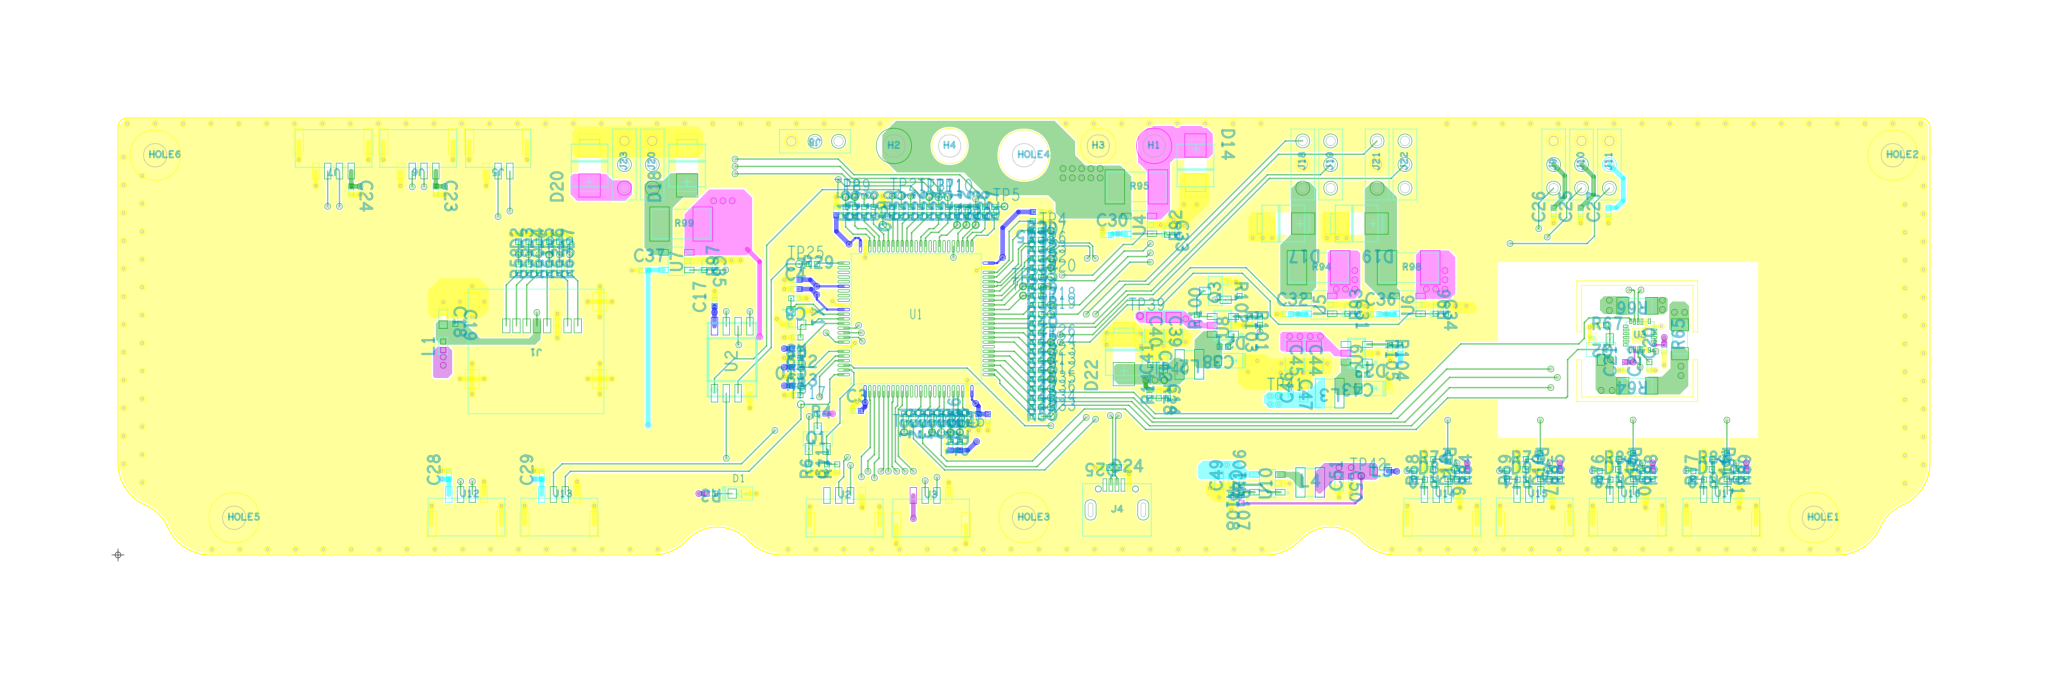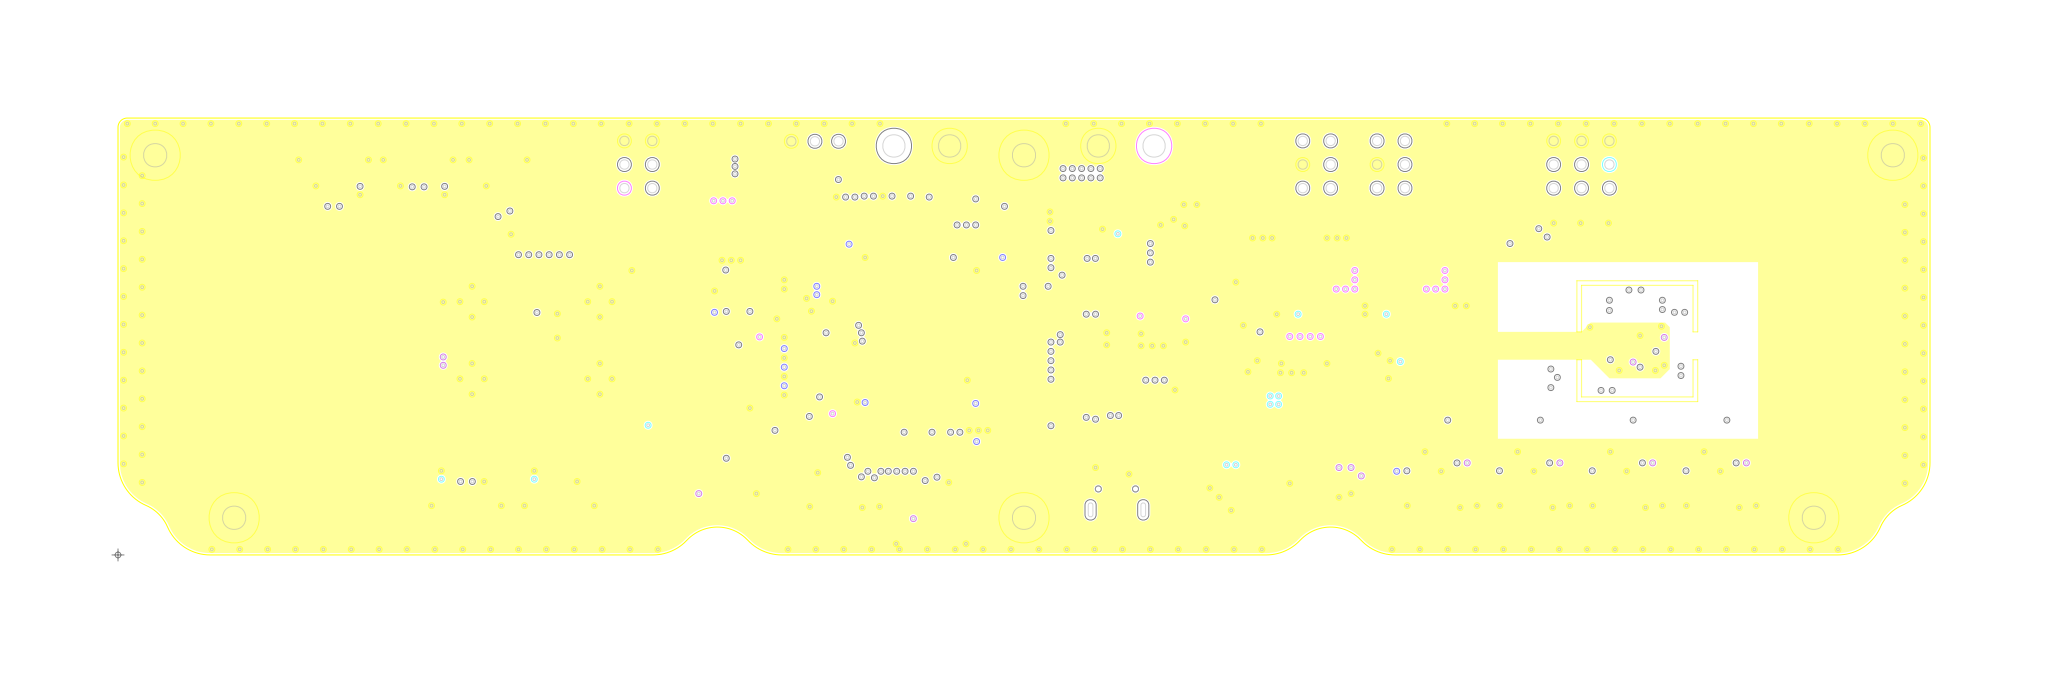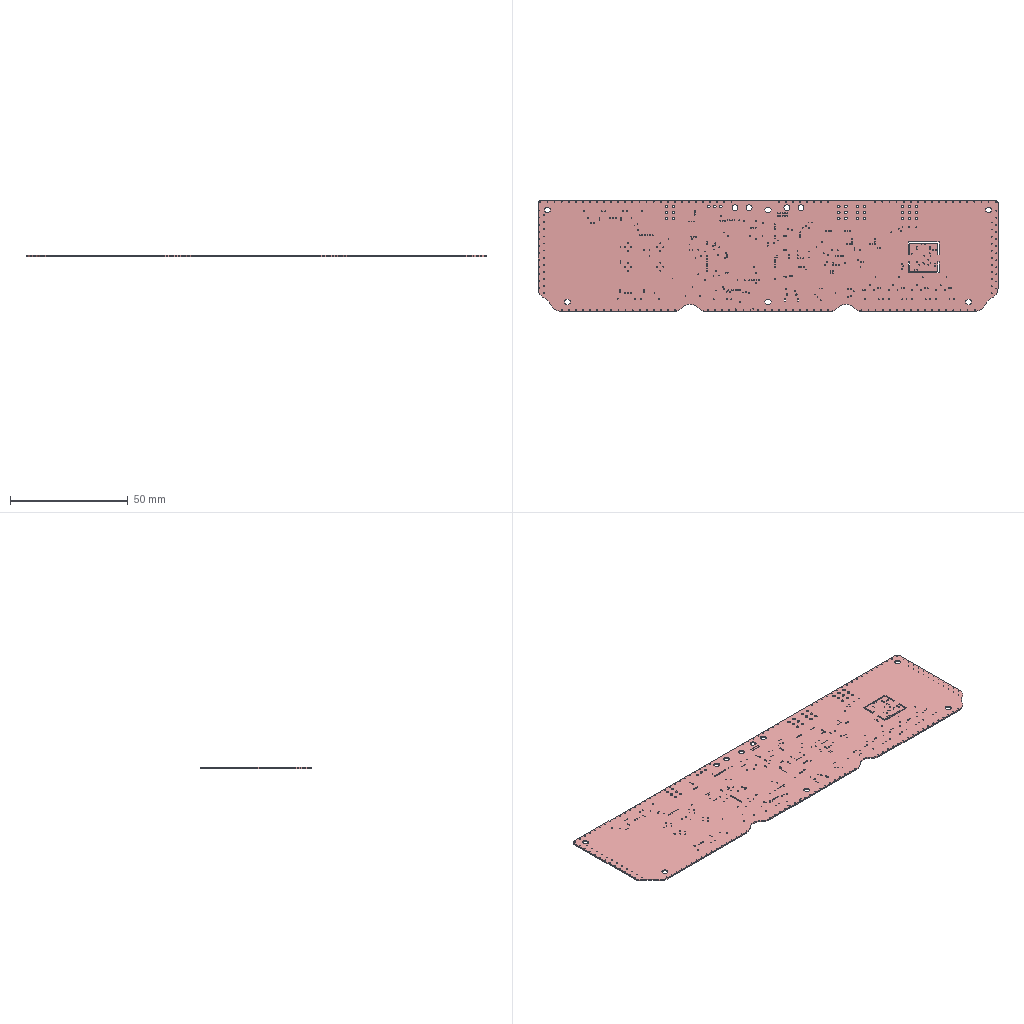Circuit board layout | Cadence Allegro | box 195 x 47 x 0.6 mm
Layer stack:
# Cadence Allegro layer stack of  (unit mm; from the constraint file cross-section; dielectric type: 0 not recorded (Allegro does not mark core vs prepreg), 3 surface material)
index,name,kind,layer,copper_thickness_mm,dielectric_type,dielectric_thickness_mm,dielectric_material,dielectric_constant
0,Top Surface,other,,,,,,
1,TOP,copper,TOP,0.0406,,,,
2,Dielectric1,dielectric,,,0,0.2032,FR-4,4.5
3,L2_GND,copper,L2_GND,0.0305,,,,
4,Dielectric2,dielectric,,,0,0.2032,FR-4,4.5
5,L3_PWR,copper,L3_PWR,0.0305,,,,
6,Dielectric3,dielectric,,,0,0.0889,FR-4,4.5
7,BOTTOM,copper,BOTTOM,0.0406,,,,
8,Bottom Surface,other,,,,,,
# drill layer pairs: low layer,high layer
drill_pair,TOP,BOTTOM
Part placement:
REFDES,COMP_VALUE,SYM_NAME,SYM_X,SYM_Y,SYM_ROTATE,SYM_MIRROR
C1,1uF,C0402,93.6,14.7,90.000,NO
C2,100nF,C0402,98.9,36.9,180.000,NO
C3,100nF,C0402,79.5,15.5,0.000,NO
C4,100nF,C0402,72.9,28.6,0.000,NO
C5,100nF,C0402,77.3,37,270.000,NO
C6,100nF,C0402,92.6,14.7,90.000,NO
C7,100nF,C0402,72.9,29.6,0.000,NO
C8,12pF,C0402,72.9,27.6,180.000,NO
C9,12pF,C0402,73,23.4,180.000,NO
C10,100nF,C0402,73,21.2,180.000,NO
C11,100nF,C0402,77.4,9.3,90.000,NO
C12,100nF,C0402,73,19.2,0.000,NO
C13,100nF,C0402,73,17.2,0.000,NO
C14,100nF,C0402,112,17.3,270.000,NO
C15,2.2uF,C0402,98.9,35.9,180.000,NO
C16,2.2uF,C0402,91.6,14.7,90.000,NO
C17,100nF,C0402,64.2,27.2,90.000,NO
C18,10uF,C0603,35,25.5,270.000,NO
C19,100nF,C0402,36.3,25.3,270.000,NO
C20,100nF,C0402,166.4,22.2,90.000,NO
C21,100nF,C0402,162.2,20.3,90.000,NO
C22,100nF,C0402,164.8,20.3,90.000,NO
C23,100nF,C0402,34.2,39.2,270.000,NO
C24,100nF,C0402,25.1,39.2,270.000,NO
C25,100nF,C0402,157.4,36.9,90.000,NO
C26,100nF,C0402,154.5,36.9,90.000,NO
C27,100nF,C0402,160.4,36.9,90.000,NO
C28,100nF,C0402,35.6,8.6,90.000,NO
C29,100nF,C0402,45.6,8.6,90.000,NO
C30,100nF,C0402,106.4,34.4,0.000,NO
C31,100nF,C0402,132.3,26.4,270.000,NO
C32,100nF,C0402,125.8,25.9,0.000,NO
C33,100nF,C0402,112.9,34.9,270.000,NO
C34,100nF,C0402,141.8,26.4,270.000,NO
C35,100nF,C0402,63.1,31.1,270.000,NO
C36,100nF,C0402,135.3,25.9,0.000,NO
C37,100nF,C0402,56.6,30.6,0.000,NO
C38,10nF,C0402,119,22.4,180.000,NO
C39,10uF,C0805,113.6,24.6,270.000,NO
C40,10uF,C0805,111.5,24.6,270.000,NO
C41,10uF,C0603,112.5,20.7,90.000,NO
C42,100nF,C0402,111.1,20.9,270.000,NO
C43,10nF,C0402,134,19.4,180.000,NO
C44,10uF,C0805,128.7,21.5,270.000,NO
C45,10uF,C0805,126.6,21.5,270.000,NO
C46,10uF,C0603,127.6,17.6,90.000,NO
C47,100nF,C0402,126.2,17.8,270.000,NO
C48,10uF,C0603,118.5,7.9,270.000,NO
C49,100nF,C0402,119.8,8,90.000,NO
C50,10uF,C0603,131.4,7.8,270.000,NO
C51,100nF,C0402,132.7,8,90.000,NO
D1,FC-DA1608HRK-620D,D0603,66.85,6.6,0.000,NO
D2,ESD5311N-2/TR,DFN1006-2L,43.1,34.1,90.000,NO
D3,ESD5311N-2/TR,DFN1006-2L,44.2,34.1,90.000,NO
D4,ESD5311N-2/TR,DFN1006-2L,45.3,34.1,90.000,NO
D5,ESD5311N-2/TR,DFN1006-2L,46.4,34.1,90.000,NO
D6,ESD5311N-2/TR,DFN1006-2L,47.5,34.1,90.000,NO
D7,ESD5311N-2/TR,DFN1006-2L,48.6,34.1,90.000,NO
D8,ESD5311N-2/TR,DFN1006-2L,141.1,9.2,0.000,NO
D9,ESD5311N-2/TR,DFN1006-2L,151.068,9.203,0.000,NO
D10,ESD5311N-2/TR,DFN1006-2L,161.055,9.203,0.000,NO
D11,ESD5311N-2/TR,DFN1006-2L,171.142,9.203,0.000,NO
D12,ESD5311N-2/TR,DFN1006-2L,143.1,8.6,90.000,NO
D13,ESD5311N-2/TR,DFN1006-2L,153.068,8.603,90.000,NO
D14,SMBJ18CA,SMBJ18CA,115.95,41.9,270.000,NO
D15,ESD5311N-2/TR,DFN1006-2L,163.055,8.603,90.000,NO
D16,ESD5311N-2/TR,DFN1006-2L,173.142,8.603,90.000,NO
D17,SMBJ18CA,SMBJ18CA,125.4,35.65,180.000,NO
D18,SMBJ18CA,SMBJ18CA,61.25,41.9,90.000,NO
D19,SMBJ18CA,SMBJ18CA,133.3,35.65,180.000,NO
D20,SMBJ18CA,SMBJ18CA,50.75,41.9,90.000,NO
D21,MBR230LSFT1G,SDO-123F_1,120,20.9,180.000,NO
D22,SMBJ5.0CA,SMBJ18CA,108.25,21.6,90.000,NO
D23,MBR230LSFT1G,SDO-123F_1,135.1,17.9,180.000,NO
D24,ESD5311N-2/TR,DFN1006-2L,108.1,9.4,0.000,NO
D25,ESD5311N-2/TR,DFN1006-2L,106.3,9.4,180.000,NO
H1,16AWG_RED,HOLE_3P8D2P4_P,111.5,44,0.000,NO
H2,16AWG_RED,HOLE_3P8D2P4_P,83.5,44,0.000,NO
H3,16AWG_BLACK,HOLE_3P8D2P4_P,105.5,44,0.000,NO
H4,16AWG_BLACK,HOLE_3P8D2P4_P,89.5,44,0.000,NO
HOLE1,T POINT R,HOLE_5P4D2P5_P,182.5,4,0.000,NO
HOLE2,T POINT R,HOLE_5P4D2P5_P,191,43,0.000,NO
HOLE3,T POINT R,HOLE_5P4D2P5_P,97.5,4,0.000,NO
HOLE4,T POINT R,HOLE_5P4D2P5_P,97.5,43,0.000,NO
HOLE5,T POINT R,HOLE_5P4D2P5_P,12.5,4,0.000,NO
HOLE6,T POINT R,HOLE_5P4D2P5_P,4,43,0.000,NO
J1,TF-102-18,TF-102-18,44.982,21.897,180.000,NO
J2,SM04B-GHS-TB,SM04B-GHS-TB,78.2,6.4,0.000,NO
J3,SM04B-GHS-TB,SM04B-GHS-TB,87.5,6.4,0.000,NO
J4,MU-103-ACY59,SMD,107.5,4.85,0.000,NO
J5,BM03B-GHS-TBT,BM03B-GHS-TBT,40.9,41.3,180.000,NO
J6,BM04B-GHS-TBT,BM04B-GHS-TBT,32.3,41.3,180.000,NO
J7,BM04B-GHS-TBT,BM04B-GHS-TBT,23.2,41.3,180.000,NO
J8,CON1X3P-T,CON1X3P-T,75,44.5,180.000,NO
J9,CON1X3P-T,CON1X3P-T,154.5,42,90.000,NO
J10,CON1X3P-T,CON1X3P-T,157.5,42,90.000,NO
J11,CON1X3P-T,CON1X3P-T,160.5,42,90.000,NO
J12,BM04B-GHS-TBT,BM04B-GHS-TBT,37.5,6.5,0.000,NO
J13,BM04B-GHS-TBT,BM04B-GHS-TBT,47.5,6.5,0.000,NO
J14,BM04B-GHS-TBT,BM04B-GHS-TBT,142.5,6.5,0.000,NO
J15,BM04B-GHS-TBT,BM04B-GHS-TBT,152.468,6.503,0.000,NO
J16,BM04B-GHS-TBT,BM04B-GHS-TBT,162.455,6.503,0.000,NO
J17,BM04B-GHS-TBT,BM04B-GHS-TBT,172.542,6.503,0.000,NO
J18,CON1X3P-T,CON1X3P-T,127.5,42,90.000,NO
J19,CON1X3P-T,CON1X3P-T,130.5,42,90.000,NO
J20,CON1X3P-T,CON1X3P-T,57.5,42,90.000,NO
J21,CON1X3P-T,CON1X3P-T,135.5,42,90.000,NO
J22,CON1X3P-T,CON1X3P-T,138.5,42,90.000,NO
J23,CON1X3P-T,CON1X3P-T,54.5,42,90.000,NO
L1,BLM15HG102SN1D,L0402,35,22.5,90.000,NO
L2,6.8uH,LVF303012-6R8M-N,115.3,20.5,180.000,NO
L3,6.8uH,LVF303012-6R8M-N,130.4,17.4,180.000,NO
L4,3.3uH,LVF303012-3R3M-N,128.3,7.8,0.000,NO
L5,BLM18PG181SN1D,L0603,135.9,9,0.000,NO
Q1,NTR4003NT1G,SOT-23_0,75.3,12.5,0.000,NO
Q2,NTR4003NT1G,SOT-23_0,159.6,22.1,180.000,NO
Q3,NTR4003NT1G,SOT-23_0,118.1,28.4,90.000,NO
R1,10K,R0402,89.6,11.7,270.000,NO
R2,10K,R0402,90.6,11.7,270.000,NO
R3,1K,R0402,63.8,6.6,180.000,NO
R4,62K,R0402,75.7,15.2,0.000,NO
R5,10K,R0402,73,22.2,180.000,NO
R6,10K,R0402,74.3,9.3,90.000,NO
R7,10K,R0402,76.3,9.3,90.000,NO
R8,0R,R0402,73,18.2,0.000,NO
R9,0R,R0402,73,20.2,0.000,NO
R10,10K,R0402,82.3,37,270.000,NO
R11,10K,R0402,90.3,37,90.000,NO
R12,10K,R0402,91.3,37,90.000,NO
R13,10K,R0402,92.3,37,90.000,NO
R14,47K,R0402,111,17.3,90.000,NO
R15,100R,R0402,78.3,37,90.000,NO
R16,100R,R0402,79.3,37,90.000,NO
R17,100R,R0402,80.3,37,90.000,NO
R18,100R,R0402,81.3,37,90.000,NO
R19,100R,R0402,83.3,37,90.000,NO
R20,22R,R0402,84.3,37,90.000,NO
R21,100R,R0402,85.3,37,90.000,NO
R22,100R,R0402,86.3,37,90.000,NO
R23,22R,R0402,87.3,37,90.000,NO
R24,100R,R0402,88.3,37,90.000,NO
R25,100R,R0402,89.3,37,90.000,NO
R26,100R,R0402,93.3,37,90.000,NO
R27,100R,R0402,94.3,37,90.000,NO
R28,10K,R0402,113,17.3,270.000,NO
R29,22R,R0402,74.8,31.3,0.000,NO
R30,100R,R0402,98.9,34.9,0.000,NO
R31,22R,R0402,98.9,33.9,0.000,NO
R32,22R,R0402,98.9,32.9,0.000,NO
R33,100R,R0402,98.9,31.9,0.000,NO
R34,100R,R0402,98.9,30.9,0.000,NO
R35,100R,R0402,98.9,29.9,0.000,NO
R36,10K,R0402,98.9,28.9,0.000,NO
R37,10K,R0402,98.9,27.9,0.000,NO
R38,100R,R0402,98.9,26.9,0.000,NO
R39,100R,R0402,98.9,25.9,0.000,NO
R40,100R,R0402,98.9,24.9,0.000,NO
R41,100R,R0402,98.9,23.9,0.000,NO
R42,22R,R0402,98.9,22.9,0.000,NO
R43,22R,R0402,98.9,21.9,0.000,NO
R44,22R,R0402,98.9,20.9,0.000,NO
R45,100R,R0402,98.9,19.9,0.000,NO
R46,100R,R0402,98.9,18.9,0.000,NO
R47,22R,R0402,98.9,17.9,0.000,NO
R48,22R,R0402,98.9,16.9,0.000,NO
R49,22R,R0402,98.9,15.9,0.000,NO
R50,22R,R0402,98.9,14.9,0.000,NO
R51,22R,R0402,84.6,14.7,270.000,NO
R52,100R,R0402,85.6,14.7,270.000,NO
R53,100R,R0402,86.6,14.7,270.000,NO
R54,100R,R0402,87.6,14.7,270.000,NO
R55,22R,R0402,88.6,14.7,270.000,NO
R56,22R,R0402,89.6,14.7,270.000,NO
R57,22R,R0402,90.6,14.7,270.000,NO
R58,10R,R0402,43.1,30.8,90.000,NO
R59,10R,R0402,44.2,30.8,90.000,NO
R60,10R,R0402,45.3,30.8,90.000,NO
R61,10R,R0402,46.4,30.8,90.000,NO
R62,10R,R0402,47.5,30.8,90.000,NO
R63,10R,R0402,48.6,30.8,90.000,NO
R64,100R,R1206,163.5,18.2,180.000,NO
R65,100R,R1206,168.1,23.2,90.000,NO
R66,100R,R1206,163.5,26.8,180.000,NO
R67,10K,R0402,159.7,24.7,0.000,NO
R68,47K,R0402,139.5,8.6,90.000,NO
R69,47K,R0402,149.468,8.603,90.000,NO
R70,20K,R0402,141.1,8.1,180.000,NO
R71,20K,R0402,151.068,8.103,180.000,NO
R72,10K,R0402,143.1,10.5,270.000,NO
R73,10K,R0402,153.068,10.503,270.000,NO
R74,47K,R0402,141.1,10.3,0.000,NO
R75,47K,R0402,151.068,10.303,0.000,NO
R76,47K,R0402,159.455,8.603,90.000,NO
R77,47K,R0402,169.542,8.603,90.000,NO
R78,20K,R0402,161.055,8.103,180.000,NO
R79,20K,R0402,171.142,8.103,180.000,NO
R80,10K,R0402,163.055,10.503,270.000,NO
R81,10K,R0402,173.142,10.503,270.000,NO
R82,47K,R0402,161.055,10.303,0.000,NO
R83,47K,R0402,171.142,10.303,0.000,NO
R84,10K,R0402,145.2,8.6,90.000,NO
R85,10K,R0402,155.168,8.603,90.000,NO
R86,10K,R0402,144.1,8.6,270.000,NO
R87,10K,R0402,154.068,8.603,270.000,NO
R88,10K,R0402,165.155,8.603,90.000,NO
R89,10K,R0402,175.242,8.603,90.000,NO
R90,10K,R0402,164.055,8.603,270.000,NO
R91,10K,R0402,174.142,8.603,270.000,NO
R92,100K,R0402,114,34.9,90.000,NO
R93,200K,R0402,133.4,26.4,90.000,NO
R94,2mR,SMD3P2X6P4,129.2,30.9,0.000,NO
R95,2mR,SMD3P2X6P4,109.6,39.6,0.000,NO
R96,200K,R0402,142.9,26.4,90.000,NO
R97,300K,R0402,64.2,31.1,90.000,NO
R98,2mR,SMD3P2X6P4,138.9,30.9,0.000,NO
R99,2mR,SMD3P2X6P4,60.6,35.6,0.000,NO
R100,100K,R0402,116.1,25.4,90.000,NO
R101,54.9K,R0402,122.9,25.2,270.000,NO
R102,10K,R0402,120.7,28.3,270.000,NO
R103,10K,R0402,121.8,25.2,270.000,NO
R104,54.9K,R0402,138,22.1,270.000,NO
R105,10K,R0402,136.9,22.1,270.000,NO
R106,10K,R0402,120.9,8,90.000,NO
R107,91K,R0402,120.9,6,270.000,NO
R108,20K,R0402,119.8,6,270.000,NO
TP1,T POINT R,TP_C1,82.3,35.5,0.000,NO
TP2,T POINT R,TP_C1,100.4,30.9,0.000,NO
TP3,T POINT R,TP_C1,100.4,31.9,0.000,NO
TP4,T POINT R,TP_C1,100.4,34.9,0.000,NO
TP5,T POINT R,TP_C1,95.4,37.5,0.000,NO
TP6,T POINT R,TP_C1,100.4,32.9,0.000,NO
TP7,T POINT R,TP_C1,100.4,33.9,0.000,NO
TP8,T POINT R,TP_C1,78.3,38.5,0.000,NO
TP9,T POINT R,TP_C1,79.3,38.5,0.000,NO
TP10,T POINT R,TP_C1,89.3,38.5,0.000,NO
TP11,T POINT R,TP_C1,88.3,38.5,0.000,NO
TP12,T POINT R,TP_C1,100.4,18.9,0.000,NO
TP13,T POINT R,TP_C1,100.4,19.9,0.000,NO
TP14,T POINT R,TP_C1,89.6,13.2,0.000,NO
TP15,T POINT R,TP_C1,90.6,13.2,0.000,NO
TP16,T POINT R,TP_C1,87.6,13.2,0.000,NO
TP17,T POINT R,TP_C1,73.5,16.2,0.000,NO
TP18,T POINT R,TP_C1,100.4,26.9,0.000,NO
TP19,T POINT R,TP_C1,100.4,25.9,0.000,NO
TP20,T POINT R,TP_C1,100.4,29.9,0.000,NO
TP21,T POINT R,TP_C1,84.3,38.6,0.000,NO
TP22,T POINT R,TP_C1,84.6,13.2,0.000,NO
TP23,T POINT R,TP_C1,100.4,20.9,0.000,NO
TP24,T POINT R,TP_C1,100.4,21.9,0.000,NO
TP25,T POINT R,TP_C1,73.3,31.3,0.000,NO
TP26,T POINT R,TP_C1,100.4,22.9,0.000,NO
TP27,T POINT R,TP_C1,97.4,27.9,0.000,NO
TP28,T POINT R,TP_C1,97.4,28.9,0.000,NO
TP29,T POINT R,TP_C1,92.3,35.5,0.000,NO
TP30,T POINT R,TP_C1,91.3,35.5,0.000,NO
TP31,T POINT R,TP_C1,90.3,35.5,0.000,NO
TP32,T POINT R,TP_C1,46.4,32.3,0.000,NO
TP33,T POINT R,TP_C1,100.4,14.9,0.000,NO
TP34,T POINT R,TP_C1,100.4,15.9,0.000,NO
TP35,T POINT R,TP_C1,100.4,17.9,0.000,NO
TP36,T POINT R,TP_C1,100.4,16.9,0.000,NO
TP37,T POINT R,TP_C1,87.3,38.5,0.000,NO
TP38,T POINT R,TP_C1,88.6,13.2,0.000,NO
TP39,T POINT R,TP_C1,110,25.7,0.000,NO
TP40,T POINT R,TP_C1,112.6,18.8,0.000,NO
TP41,T POINT R,TP_C1,124.9,17.1,0.000,NO
TP42,T POINT R,TP_C1,133.8,8.5,0.000,NO
U1,STM32F745VGT6,LQFP-100,85.9,25.4,0.000,NO
U2,W25Q128JV,SOIC-8-208MIL,66.097,21.001,90.000,NO
U3,MPU6500,QFN,163.8,23.6,0.000,NO
U4,SGM8198,SOT-23_5,109.9,35.5,90.000,NO
U5,SGM8198,SOT-23_5,129.3,26.9,90.000,NO
U6,SGM8198,SOT-23_5,138.8,26.9,90.000,NO
U7,SGM8198,SOT-23_5,60.1,31.6,90.000,NO
U8,RT8259GJ6,TSOT-23-6,118.9,24.7,90.000,NO
U9,RT8259GJ6,TSOT-23-6,133.3,21.7,90.000,NO
U10,RT8096CHGJ5,TSOT-23-5,123.7,7.7,90.000,NO
X1,YSX211SL,SMD2016,73,25.5,270.000,NO
Pad and via stacks:
# Allegro (Cadence) via spans and padstacks; design units: ("millimeters" 4 10000)
# via spans: padstack,start_layer,end_layer,net_example,count
VIA12-BGA,ETCH/TOP,ETCH/BOTTOM,GND,497
# Allegro padstack definitions: name,start_layer,end_layer,drill,plating,holeType,type
SMDS0P55,"ETCH/TOP","ETCH/TOP",0.0,"PLATED","none","smd"
TS0P8128_B,"ETCH/BOTTOM","ETCH/BOTTOM",0.0,"PLATED","none","smd"
SMD1P0X0P9,"ETCH/TOP","ETCH/TOP",0.0,"PLATED","none","smd"
SMD0P25X0P7,"ETCH/TOP","ETCH/TOP",0.0,"PLATED","none","smd"
SMD1P6X1P7,"ETCH/TOP","ETCH/TOP",0.0,"PLATED","none","smd"
SMD0P35X0P7,"ETCH/TOP","ETCH/TOP",0.0,"PLATED","none","smd"
SMD0P5X0P725,"ETCH/TOP","ETCH/TOP",0.0,"PLATED","none","smd"
SMD0P4X0P8,"ETCH/TOP","ETCH/TOP",0.0,"PLATED","none","smd"
SMD0P889X0P8128,"ETCH/TOP","ETCH/TOP",0.0,"PLATED","none","smd"
SMD0P25X1P45,"ETCH/TOP","ETCH/TOP",0.0,"PLATED","none","smd"
SMD0P45X1P45,"ETCH/TOP","ETCH/TOP",0.0,"PLATED","none","smd"
SMD0P25X1P7,"ETCH/TOP","ETCH/TOP",0.0,"PLATED","none","smd"
SMD0P45X1P7,"ETCH/TOP","ETCH/TOP",0.0,"PLATED","none","smd"
SMDC0P762,"ETCH/TOP","ETCH/TOP",0.0,"NON_PLATED","none","smd"
SMD1P6X1P1,"ETCH/TOP","ETCH/TOP",0.0,"PLATED","none","smd"
SMDS3P7_NP,"ETCH/TOP","ETCH/TOP",0.0,"PLATED","none","smd"
SMD0P21X0P85,"ETCH/TOP","ETCH/TOP",0.0,"PLATED","none","smd"
SMD1P1X2P9,"ETCH/TOP","ETCH/TOP",0.0,"PLATED","none","smd"
SMD0P65X1P6,"ETCH/TOP","ETCH/TOP",0.0,"PLATED","none","smd"
SMD0P25X0P6,"ETCH/TOP","ETCH/TOP",0.0,"PLATED","none","smd"
SMDS1P6,"ETCH/TOP","ETCH/TOP",0.0,"PLATED","none","smd"
SMDC0P5,"ETCH/TOP","ETCH/TOP",0.0,"PLATED","none","smd"
AR0P55X0P50,"ETCH/TOP","ETCH/TOP",0.0,"PLATED","none","smd"
SMD1P7X2P5,"ETCH/TOP","ETCH/TOP",0.0,"PLATED","none","smd"
SMDS0P6,"ETCH/TOP","ETCH/TOP",0.0,"PLATED","none","smd"
SMDS0P8,"ETCH/TOP","ETCH/TOP",0.0,"PLATED","none","smd"
SMDC1P016_2P032_NP,"ETCH/TOP","ETCH/TOP",0.0,"PLATED","none","smd"
SMD1P6X2P8,"ETCH/TOP","ETCH/TOP",0.0,"PLATED","none","smd"
SMDC0P3,"ETCH/TOP","ETCH/TOP",0.0,"PLATED","none","smd"
SMDF1P6X0P6,"ETCH/TOP","ETCH/TOP",0.0,"PLATED","none","smd"
SMD43_10,"ETCH/TOP","ETCH/TOP",0.0,"PLATED","none","smd"
SMD28_10,"ETCH/TOP","ETCH/TOP",0.0,"PLATED","none","smd"
SMD025X08,"ETCH/TOP","ETCH/TOP",0.0,"PLATED","none","smd"
SMD1R1X2R75,"ETCH/TOP","ETCH/TOP",0.0,"PLATED","none","smd"
SMD10_28,"ETCH/TOP","ETCH/TOP",0.0,"NON_PLATED","none","smd"
SMD10_43,"ETCH/TOP","ETCH/TOP",0.0,"PLATED","none","smd"
SMD10_11,"ETCH/TOP","ETCH/TOP",0.0,"NON_PLATED","none","smd"
SMD1P6X1P3,"ETCH/TOP","ETCH/TOP",0.0,"PLATED","none","smd"
SMD1P4X1P2,"ETCH/TOP","ETCH/TOP",0.0,"PLATED","none","smd"
PAD_OCT_SMD_20,"ETCH/TOP","ETCH/TOP",0.0,"PLATED","none","smd"
SMD0P7X0P22,"ETCH/TOP","ETCH/TOP",0.0,"PLATED","none","smd"
SMD1P4X2P8,"ETCH/TOP","ETCH/TOP",0.0,"PLATED","none","smd"
SMD1P8X1P3,"ETCH/TOP","ETCH/TOP",0.0,"PLATED","none","smd"
SMD2P54X2P794,"ETCH/TOP","ETCH/TOP",0.0,"PLATED","none","smd"
SMD1P2X0P8,"ETCH/TOP","ETCH/TOP",0.0,"PLATED","none","smd"
SMD0P2X0P7,"ETCH/TOP","ETCH/TOP",0.0,"PLATED","none","smd"
SMD0P4X0P75,"ETCH/TOP","ETCH/TOP",0.0,"PLATED","none","smd"
SMD3P5X1P5,"ETCH/TOP","ETCH/TOP",0.0,"PLATED","none","smd"
SMD0P6X0P85,"ETCH/TOP","ETCH/TOP",0.0,"PLATED","none","smd"
SMD0P3X0P85,"ETCH/TOP","ETCH/TOP",0.0,"PLATED","none","smd"
SMD1P5X4P7,"ETCH/TOP","ETCH/TOP",0.0,"PLATED","none","smd"
SMD0P75X1P1,"ETCH/TOP","ETCH/TOP",0.0,"PLATED","none","smd"
SMD0P9X1P2,"ETCH/TOP","ETCH/TOP",0.0,"PLATED","none","smd"
SMD0P9X2P0,"ETCH/TOP","ETCH/TOP",0.0,"PLATED","none","smd"
SMDS1P3,"ETCH/TOP","ETCH/TOP",0.0,"PLATED","none","smd"
SMD0P7X2P0,"ETCH/TOP","ETCH/TOP",0.0,"PLATED","none","smd"
SMD2P5X2P3,"ETCH/TOP","ETCH/TOP",0.0,"PLATED","none","smd"
SMD1P0X0P8,"ETCH/TOP","ETCH/TOP",0.0,"PLATED","none","smd"
SMD1P9X0P7,"ETCH/TOP","ETCH/TOP",0.0,"PLATED","none","smd"
SMD0P6X1P0,"ETCH/TOP","ETCH/TOP",0.0,"PLATED","none","smd"
SMD1P06X0P65,"ETCH/TOP","ETCH/TOP",0.0,"PLATED","none","smd"
SMD0P25X0P5,"ETCH/TOP","ETCH/TOP",0.0,"PLATED","none","smd"
SMD0P2X0P6,"ETCH/TOP","ETCH/TOP",0.0,"PLATED","none","smd"
C0_27X1_27,"ETCH/TOP","ETCH/TOP",0.0,"NON_PLATED","none","smd"
SMD2P1X3P68,"ETCH/TOP","ETCH/TOP",0.0,"PLATED","none","smd"
SMD1P0X3P2,"ETCH/TOP","ETCH/TOP",0.0,"PLATED","none","smd"
SMD0P25X0P35,"ETCH/TOP","ETCH/TOP",0.0,"PLATED","none","smd"
SMD0P7X1P7,"ETCH/TOP","ETCH/TOP",0.0,"PLATED","none","smd"
SMD1P0X2P7,"ETCH/TOP","ETCH/TOP",0.0,"PLATED","none","smd"
SMD0P8X1P5,"ETCH/TOP","ETCH/TOP",0.0,"PLATED","none","smd"
SMD1P5X2P0,"ETCH/TOP","ETCH/TOP",0.0,"PLATED","none","smd"
SMD0P4X1P35,"ETCH/TOP","ETCH/TOP",0.0,"PLATED","none","smd"
VIA16D08,"ETCH/TOP","ETCH/BOTTOM",0.2032,"PLATED","circle_drill","through"
NTHC0P8,"ETCH/TOP","ETCH/BOTTOM",0.8001,"NON_PLATED","circle_drill","through"
THC4P0D2P2,"ETCH/TOP","ETCH/BOTTOM",2.2,"PLATED","circle_drill","through"
THC1P4D0P9,"ETCH/TOP","ETCH/BOTTOM",0.8999,"PLATED","circle_drill","through"
THS1P0D0P5,"ETCH/TOP","ETCH/BOTTOM",0.5001,"PLATED","circle_drill","through"
THC1P0D0P5,"ETCH/TOP","ETCH/BOTTOM",0.5001,"PLATED","circle_drill","through"
THC4P0D3P0,"ETCH/TOP","ETCH/BOTTOM",3.0,"PLATED","circle_drill","through"
H0300,"ETCH/TOP","ETCH/BOTTOM",3.0,"NON_PLATED","circle_drill","through"
H0150,"ETCH/TOP","ETCH/BOTTOM",1.5,"NON_PLATED","circle_drill","through"
THC4P5D2P2,"ETCH/TOP","ETCH/BOTTOM",2.2,"PLATED","circle_drill","through"
THS1P3D0P8,"ETCH/TOP","ETCH/BOTTOM",0.8,"PLATED","circle_drill","through"
THC1P3D0P8,"ETCH/TOP","ETCH/BOTTOM",0.8,"PLATED","circle_drill","through"
THS1P651D1P016,"ETCH/TOP","ETCH/BOTTOM",1.016,"PLATED","circle_drill","through"
THC1P651D1P016,"ETCH/TOP","ETCH/BOTTOM",1.016,"PLATED","circle_drill","through"
THC4P2D2P2,"ETCH/TOP","ETCH/BOTTOM",2.2,"PLATED","circle_drill","through"
VIA12-BGA,"ETCH/TOP","ETCH/BOTTOM",0.3048,"PLATED","circle_drill","through"
THS1P4D0P9,"ETCH/TOP","ETCH/BOTTOM",0.9,"PLATED","circle_drill","through"
THC2P54D1P8,"ETCH/TOP","ETCH/BOTTOM",1.8,"PLATED","circle_drill","through"
HOLE3P2,"ETCH/TOP","ETCH/BOTTOM",3.2,"NON_PLATED","circle_drill","through"
HOLE0P65,"ETCH/TOP","ETCH/BOTTOM",0.65,"NON_PLATED","circle_drill","through"
THO2P1X1P0D1P7X0P6,"ETCH/TOP","ETCH/BOTTOM",0.6,"PLATED","oval slot","through"
THO1P6X1P0D1P2X0P6,"ETCH/TOP","ETCH/BOTTOM",0.6,"PLATED","oval slot","through"
NTHC0P7,"ETCH/TOP","ETCH/BOTTOM",0.7,"NON_PLATED","circle_drill","through"
THC1P524D0P8,"ETCH/TOP","ETCH/BOTTOM",0.8,"PLATED","circle_drill","through"
THC5P0D2P5,"ETCH/TOP","ETCH/BOTTOM",2.5,"PLATED","circle_drill","through"
THC3P5D2P4,"ETCH/TOP","ETCH/BOTTOM",2.4,"PLATED","circle_drill","through"
THC1P5D1P0,"ETCH/TOP","ETCH/BOTTOM",1.0,"PLATED","circle_drill","through"
THO2P2X1P2D1P5X0P5,"ETCH/TOP","ETCH/BOTTOM",0.5,"PLATED","oval slot","through"
THC3P8D2P4,"ETCH/TOP","ETCH/BOTTOM",2.4,"PLATED","circle_drill","through"
THC5P4D2P5,"ETCH/TOP","ETCH/BOTTOM",2.5,"PLATED","circle_drill","through"
Design rules, without the lines most boards share, first 16 of 31 lines:
# Cadence Allegro design rules of  (from the Constraint Manager export constraints.dcfx, design unit mm; typed fields in mm)
# columns: name | kind | enabled | priority | scope1 | scope2 | descriptor | typed fields (field=value)
# Allegro precedence (priority 1 wins): 1 Region class-to-class, 2 Region class, 3 Region, 4 class-to-class, 5 DiffPair/Bus/NetGroup override, 6 NetClass, 7 constraint set (CSet) default
# per-layer values are written LAYER=value in the descriptor and LAYER:mm in the typed field; a maximum of 0 means no limit set
# --- net classes (and buses / net groups) ---
DIFF100 | NetClass | enabled | 6 | no members | All | Net Class (members: 0) overrides: (DIFFP_PHASE_TOL=0.127 mm) |  diffp_phase_tol=0.127mm
MIPI | NetClass | enabled | 6 | no members | All | Net Class (members: 0) |
DEFAULT | NetClass | enabled | 6 | no members | All | Net Class (members: 0) |
15 | NetClass | enabled | 6 | no members | All | Net Class (members: 0) |
20 | NetClass | enabled | 6 | no members | All | Net Class (members: 0) |
# --- track widths, neck and differential-pair gap (physical constraint sets) ---
DEFAULT | PhysicalCSet | enabled | 7 | Design default | All | Physical Constraint (Min Line Width=0.16mm) (Max Line Width=0mm) (Min Neck Width=0.16mm) (Max Neck Length=0.16mm) (DiffPair Primary Gap=0.16mm) (DiffPair Neck Gap=0.16mm) (DiffPair Min Space=0.16mm) (DiffPair Coupled +Tol=0mm) (DiffPair Coupled -Tol=0mm) (Min BB Via Stagger=0.16mm) (Max BB Via Stagger=0.16mm) (T-junctions=ANYWHERE) (Pad-pad direct connect=ALL_ALLOWED) (Allowed vias=VIA12-BGA) | min_line_width=0.16 min_neck_width=0.16 min_bvia_stagger=0.16 max_bvia_stagger=0.16 ts_allowed=ANYWHERE diffp_primary_gap=0.16 diffp_neck_gap=0.16 max_line_width=0 maximum_neck_length=0.16 pad_pad_direct_connect=ALL_ALLOWED allow_on_etch_subclass=TRUE diffp_coupled_plus=0 diffp_coupled_minus=0 diffp_min_space=0.16 vias=VIA12-BGA
# --- clearances: line / pad / via / shape / hole (spacing constraint sets) ---
DEFAULT | SpacingCSet | enabled | 7 | Design default; Region(1): DEFAULT | All | Clearance Constraint (Line-Line=0.16mm) (Line-SMD Pad=0.16mm) (Line-Thru Pin=0.16mm) (Line-Via=0.16mm) (Line-Shape=0.16mm) (SMD Pad-SMD Pad=0.15mm) (Thru Pin-Thru Pin=0.16mm) (Thru Pin-SMD Pad=0.16mm) (SMD Pad-Via=0.16mm) (Thru Pin-Via=0.16mm) (Via-Via=0.16mm) (Shape-SMD Pad=0.16mm) (Shape-Thru Pin=0.16mm) (Shape-Via=0.16mm) (Shape-Shape=0.16mm) (Hole-Hole=0.16mm) (Hole-Line=0.16mm) (Hole-Shape=0.16mm) (BB Via-BB Via=0.16mm) (uVia-uVia=0.16mm) | thrupin_to_thrupin_spacing=0.16 thrupin_to_smdpin_spacing=0.16 thrupin_to_thruvia_spacing=0.16 line_to_thrupin_spacing=0.16 thrupin_to_shape_spacing=0.16 smdpin_to_smdpin_spacing=0.15 smdpin_to_thruvia_spacing=0.16 line_to_smdpin_spacing=0.16 shape_to_smdpin_spacing=0.16 thruvia_to_thruvia_spacing=0.16 line_to_thruvia_spacing=0.16 shape_to_thruvia_spacing=0.16 line_to_line_spacing=0.16 line_to_shape_spacing=0.16 shape_to_shape_spacing=0.16 bbv_to_bbv_spacing=0.16 bbv_to_thrupin_spacing=0.16 bbv_to_smdpin_spacing=0.16 bbv_to_thruvia_spacing=0.16 bbv_to_line_spacing=0.16 bbv_to_shape_spacing=0.16 bbv_to_testpin_spacing=0.16 bbv_to_testvia_spacing=0.16 testpin_to_testpin_spacing=0.16 testpin_to_thrupin_spacing=0.16 smdpin_to_testpin_spacing=0.16 testpin_to_thruvia_spacing=0.16 testpin_to_testvia_spacing=0.16 line_to_testpin_spacing=0.16 shape_to_testpin_spacing=0.16 testvia_to_testvia_spacing=0.16 testvia_to_thrupin_spacing=0.16 smdpin_to_testvia_spacing=0.16 testvia_to_thruvia_spacing=0.16 line_to_testvia_spacing=0.16 shape_to_testvia_spacing=0.16 bondpad_to_bondpad_spacing=0.16 thrupin_to_bondpad_spacing=0.16 smdpin_to_bondpad_spacing=0.16 bondpad_to_thruvia_spacing=0.16 bondpad_to_line_spacing=0.16 bondpad_to_shape_spacing=0.16 bondpad_to_bbv_spacing=0.16 bondpad_to_testpin_spacing=0.16 bondpad_to_testvia_spacing=0.16 min_bvia_gap=0.254 hole_to_pin_spacing=0.16 hole_to_via_spacing=0.16 hole_to_line_spacing=0.16 hole_to_shape_spacing=0.16 hole_to_hole_spacing=0.16 mvia_to_mvia_spacing=0.16 mvia_to_thrupin_spacing=0.16 mvia_to_smdpin_spacing=0.16 mvia_to_thruvia_spacing=0.16 mvia_to_bbv_spacing=0.16 mvia_to_line_spacing=0.16 mvia_to_shape_spacing=0.16 mvia_to_testpin_spacing=0.16 mvia_to_testvia_spacing=0.16 bondpad_to_mvia_spacing=0.16 bondpad_to_bondpad_diffp_spc=0.127
DEFAULT | SameNetSpacingCSet | enabled | 7 | Design default | All | Same-Net Clearance (Line-Line=0.127mm) (Line-SMD Pad=0.127mm) (Line-Thru Pin=0.127mm) (Line-Via=0.127mm) (Line-Shape=0.127mm) (SMD Pad-SMD Pad=0.127mm) (Thru Pin-Thru Pin=0.127mm) (Thru Pin-SMD Pad=0.127mm) (SMD Pad-Via=0.0762mm) (Thru Pin-Via=0.127mm) (Via-Via=0.127mm) (Shape-SMD Pad=0.127mm) (Shape-Thru Pin=0.127mm) (Shape-Via=0.127mm) (Shape-Shape=0.127mm) (Hole-Hole=0.2032mm) (Hole-Line=0.2032mm) (Hole-Shape=0.2032mm) (BB Via-BB Via=0.127mm) (uVia-uVia=0.127mm) | sn_thrupin_to_thrupin_spacing=0.127 sn_thrupin_to_smdpin_spacing=0.127 sn_thrupin_to_thruvia_spacing=0.127 sn_line_to_thrupin_spacing=0.127 sn_thrupin_to_shape_spacing=0.127 sn_smdpin_to_smdpin_spacing=0.127 sn_smdpin_to_thruvia_spacing=0.0762 sn_line_to_smdpin_spacing=0.127 sn_shape_to_smdpin_spacing=0.127 sn_thruvia_to_thruvia_spacing=0.127 sn_line_to_thruvia_spacing=0.127 sn_shape_to_thruvia_spacing=0.127 sn_line_to_line_spacing=0.127 sn_line_to_shape_spacing=0.127 sn_shape_to_shape_spacing=0.127 sn_bbv_to_bbv_spacing=0.127 sn_bbv_to_thrupin_spacing=0.127 sn_bbv_to_smdpin_spacing=0.127 sn_bbv_to_thruvia_spacing=0.127 sn_bbv_to_line_spacing=0.127 sn_bbv_to_shape_spacing=0.127 sn_bbv_to_testpin_spacing=0.127 sn_bbv_to_testvia_spacing=0.127 sn_testpin_to_testpin_spacing=0.127 sn_testpin_to_thrupin_spacing=0.127 sn_smdpin_to_testpin_spacing=0.127 sn_testpin_to_thruvia_spacing=0.127 sn_testpin_to_testvia_spacing=0.127 sn_line_to_testpin_spacing=0.127 sn_shape_to_testpin_spacing=0.127 sn_testvia_to_testvia_spacing=0.127 sn_testvia_to_thrupin_spacing=0.127 sn_smdpin_to_testvia_spacing=0.127 sn_testvia_to_thruvia_spacing=0.127 sn_line_to_testvia_spacing=0.127 sn_shape_to_testvia_spacing=0.127 sn_bondpad_to_bondpad_spacing=0.127 sn_thrupin_to_bondpad_spacing=0.127 sn_smdpin_to_bondpad_spacing=0.127 sn_bondpad_to_thruvia_spacing=0.127 sn_bondpad_to_line_spacing=0.127 sn_bondpad_to_shape_spacing=0.127 sn_bondpad_to_bbv_spacing=0.127 sn_bondpad_to_testpin_spacing=0.127 sn_bondpad_to_testvia_spacing=0.127 same_net=TRUE sn_hole_to_pin_spacing=0.2032 sn_hole_to_via_spacing=0.2032 sn_hole_to_line_spacing=0.2032 sn_hole_to_shape_spacing=0.2032 sn_hole_to_hole_spacing=0.2032 sn_mvia_to_mvia_spacing=0.127 sn_mvia_to_thrupin_spacing=0.127 sn_mvia_to_smdpin_spacing=0.127 sn_mvia_to_thruvia_spacing=0.127 sn_mvia_to_bbv_spacing=0.127 sn_mvia_to_line_spacing=0.127 sn_mvia_to_shape_spacing=0.127 sn_mvia_to_testpin_spacing=0.127 sn_mvia_to_testvia_spacing=0.127 sn_bondpad_to_mvia_spacing=0.127
0.65BGA | Region | enabled | 3 | Region 0.65BGA | All | Region Constraint  |